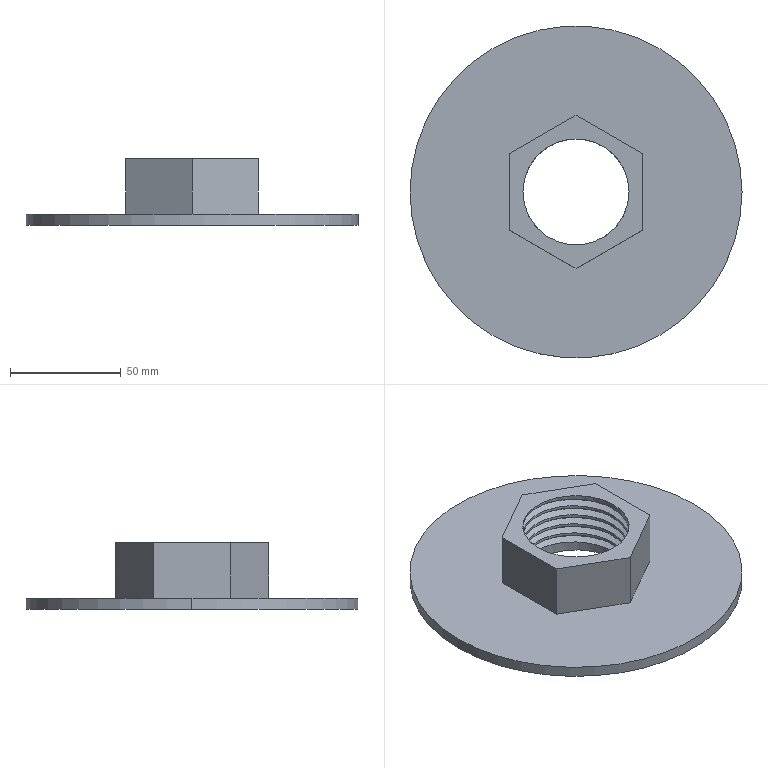Part | SolidWorks | features ICE 2, Cut 1, Extrusion 1, SweepThread 1 | 1 solid | 28 faces | box 150 x 150 x 30 mm | volume 107137 mm3 | cylinder 14 | plane 11 | spline 3 | commonest cylinder face diameters 48 x12 150 x2